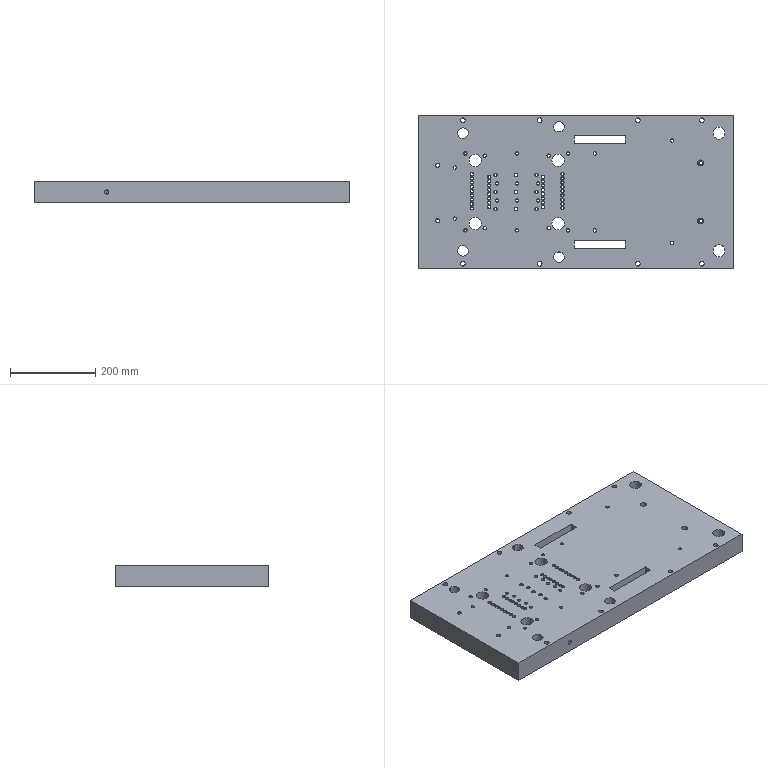Part | STEP file | 1 solid | 388 faces | box 740 x 360 x 50 mm | volume 12464392 mm3 | cone 181 | cylinder 177 | plane 30 | commonest cylinder face diameters 6.8 x67 1 x42 5 x18 8.01 x10 11 x8 17 x8